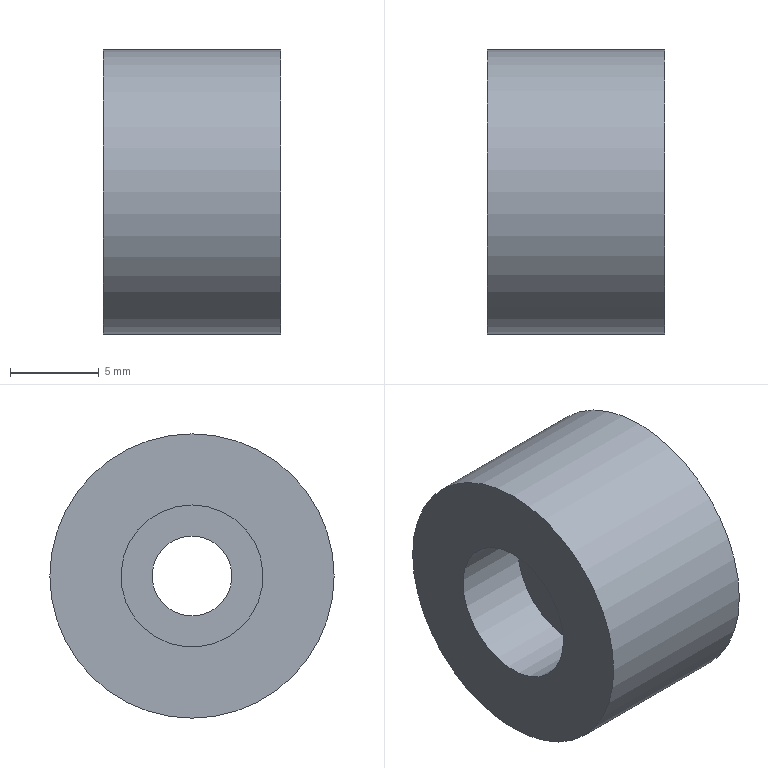Part | NX | 1 solid | 6 faces | box 10 x 16 x 16 mm | volume 1700 mm3 | plane 3 | cylinder 3 | commonest cylinder face diameters 4.5 x1 8 x1 16 x1
STEP:
#1=CARTESIAN_POINT('',(0.,0.,8.));
#2=VERTEX_POINT('',#1);
#3=CARTESIAN_POINT('',(0.,0.,0.));
#4=DIRECTION('',(-1.,0.,0.));
#5=DIRECTION('',(0.,0.,1.));
#6=AXIS2_PLACEMENT_3D('',#3,#4,#5);
#7=CIRCLE('',#6,8.);
#8=EDGE_CURVE('',#2,#2,#7,.T.);
#9=ORIENTED_EDGE('',*,*,#8,.T.);
#10=EDGE_LOOP('',(#9));
#11=FACE_BOUND('',#10,.T.);
#12=CARTESIAN_POINT('',(0.,0.,4.));
#13=VERTEX_POINT('',#12);
#14=CARTESIAN_POINT('',(0.,0.,0.));
#15=DIRECTION('',(-1.,0.,0.));
#16=DIRECTION('',(0.,0.,1.));
#17=AXIS2_PLACEMENT_3D('',#14,#15,#16);
#18=CIRCLE('',#17,4.);
#19=EDGE_CURVE('',#13,#13,#18,.T.);
#20=ORIENTED_EDGE('',*,*,#19,.F.);
#21=EDGE_LOOP('',(#20));
#22=FACE_BOUND('',#21,.T.);
#23=CARTESIAN_POINT('',(0.,0.,-4.));
#24=DIRECTION('',(-1.,0.,0.));
#25=DIRECTION('',(0.,0.,-1.));
#26=AXIS2_PLACEMENT_3D('',#23,#24,#25);
#27=PLANE('',#26);
#28=ADVANCED_FACE('',(#11,#22),#27,.T.);
#29=CARTESIAN_POINT('',(10.,0.,8.));
#30=VERTEX_POINT('',#29);
#31=CARTESIAN_POINT('',(10.,0.,0.));
#32=DIRECTION('',(-1.,0.,0.));
#33=DIRECTION('',(0.,0.,1.));
#34=AXIS2_PLACEMENT_3D('',#31,#32,#33);
#35=CIRCLE('',#34,8.);
#36=EDGE_CURVE('',#30,#30,#35,.T.);
#37=ORIENTED_EDGE('',*,*,#36,.T.);
#38=EDGE_LOOP('',(#37));
#39=FACE_BOUND('',#38,.T.);
#40=ORIENTED_EDGE('',*,*,#8,.F.);
#41=EDGE_LOOP('',(#40));
#42=FACE_BOUND('',#41,.T.);
#43=CARTESIAN_POINT('',(10.,0.,0.));
#44=DIRECTION('',(-1.,0.,0.));
#45=DIRECTION('',(0.,0.,-1.));
#46=AXIS2_PLACEMENT_3D('',#43,#44,#45);
#47=CYLINDRICAL_SURFACE('',#46,8.);
#48=ADVANCED_FACE('',(#39,#42),#47,.T.);
#49=CARTESIAN_POINT('',(10.,0.,2.25));
#50=VERTEX_POINT('',#49);
#51=CARTESIAN_POINT('',(10.,0.,0.));
#52=DIRECTION('',(-1.,0.,0.));
#53=DIRECTION('',(0.,0.,1.));
#54=AXIS2_PLACEMENT_3D('',#51,#52,#53);
#55=CIRCLE('',#54,2.25);
#56=EDGE_CURVE('',#50,#50,#55,.T.);
#57=ORIENTED_EDGE('',*,*,#56,.T.);
#58=EDGE_LOOP('',(#57));
#59=FACE_BOUND('',#58,.T.);
#60=ORIENTED_EDGE('',*,*,#36,.F.);
#61=EDGE_LOOP('',(#60));
#62=FACE_BOUND('',#61,.T.);
#63=CARTESIAN_POINT('',(10.,0.,-8.));
#64=DIRECTION('',(1.,0.,0.));
#65=DIRECTION('',(0.,0.,1.));
#66=AXIS2_PLACEMENT_3D('',#63,#64,#65);
#67=PLANE('',#66);
#68=ADVANCED_FACE('',(#59,#62),#67,.T.);
#69=CARTESIAN_POINT('',(4.4,0.,2.25));
#70=VERTEX_POINT('',#69);
#71=CARTESIAN_POINT('',(4.4,0.,0.));
#72=DIRECTION('',(-1.,0.,0.));
#73=DIRECTION('',(0.,0.,1.));
#74=AXIS2_PLACEMENT_3D('',#71,#72,#73);
#75=CIRCLE('',#74,2.25);
#76=EDGE_CURVE('',#70,#70,#75,.T.);
#77=ORIENTED_EDGE('',*,*,#76,.T.);
#78=EDGE_LOOP('',(#77));
#79=FACE_BOUND('',#78,.T.);
#80=ORIENTED_EDGE('',*,*,#56,.F.);
#81=EDGE_LOOP('',(#80));
#82=FACE_BOUND('',#81,.T.);
#83=CARTESIAN_POINT('',(10.,0.,0.));
#84=DIRECTION('',(-1.,0.,0.));
#85=DIRECTION('',(0.,0.,-1.));
#86=AXIS2_PLACEMENT_3D('',#83,#84,#85);
#87=CYLINDRICAL_SURFACE('',#86,2.25);
#88=ADVANCED_FACE('',(#79,#82),#87,.F.);
#89=CARTESIAN_POINT('',(4.4,0.,4.));
#90=VERTEX_POINT('',#89);
#91=CARTESIAN_POINT('',(4.4,0.,0.));
#92=DIRECTION('',(-1.,0.,0.));
#93=DIRECTION('',(0.,0.,1.));
#94=AXIS2_PLACEMENT_3D('',#91,#92,#93);
#95=CIRCLE('',#94,4.);
#96=EDGE_CURVE('',#90,#90,#95,.T.);
#97=ORIENTED_EDGE('',*,*,#96,.T.);
#98=EDGE_LOOP('',(#97));
#99=FACE_BOUND('',#98,.T.);
#100=ORIENTED_EDGE('',*,*,#76,.F.);
#101=EDGE_LOOP('',(#100));
#102=FACE_BOUND('',#101,.T.);
#103=CARTESIAN_POINT('',(4.4,0.,-2.25));
#104=DIRECTION('',(-1.,0.,0.));
#105=DIRECTION('',(0.,0.,-1.));
#106=AXIS2_PLACEMENT_3D('',#103,#104,#105);
#107=PLANE('',#106);
#108=ADVANCED_FACE('',(#99,#102),#107,.T.);
#109=ORIENTED_EDGE('',*,*,#19,.T.);
#110=EDGE_LOOP('',(#109));
#111=FACE_BOUND('',#110,.T.);
#112=ORIENTED_EDGE('',*,*,#96,.F.);
#113=EDGE_LOOP('',(#112));
#114=FACE_BOUND('',#113,.T.);
#115=CARTESIAN_POINT('',(10.,0.,0.));
#116=DIRECTION('',(-1.,0.,0.));
#117=DIRECTION('',(0.,0.,-1.));
#118=AXIS2_PLACEMENT_3D('',#115,#116,#117);
#119=CYLINDRICAL_SURFACE('',#118,4.);
#120=ADVANCED_FACE('',(#111,#114),#119,.F.);
#121=CLOSED_SHELL('',(#28,#48,#68,#88,#108,#120));
#122=MANIFOLD_SOLID_BREP('',#121);
#123=(LENGTH_UNIT()NAMED_UNIT(*)SI_UNIT(.MILLI.,.METRE.));
#124=UNCERTAINTY_MEASURE_WITH_UNIT(LENGTH_MEASURE(0.00002),#123,'','');
#125=(NAMED_UNIT(*)PLANE_ANGLE_UNIT()SI_UNIT($,.RADIAN.));
#126=PLANE_ANGLE_MEASURE_WITH_UNIT(PLANE_ANGLE_MEASURE(0.01745),#125);
#127=DIMENSIONAL_EXPONENTS(0.,0.,0.,0.,0.,0.,0.);
#128=(CONVERSION_BASED_UNIT('DEGREE',#126)NAMED_UNIT(#127)PLANE_ANGLE_UNIT());
#129=(NAMED_UNIT(*)SI_UNIT($,.STERADIAN.)SOLID_ANGLE_UNIT());
#130=(GEOMETRIC_REPRESENTATION_CONTEXT(3)GLOBAL_UNCERTAINTY_ASSIGNED_CONTEXT((#124))GLOBAL_UNIT_ASSIGNED_CONTEXT((#123,#128,#129))REPRESENTATION_CONTEXT('',''));
#131=ADVANCED_BREP_SHAPE_REPRESENTATION('',(#122),#130);